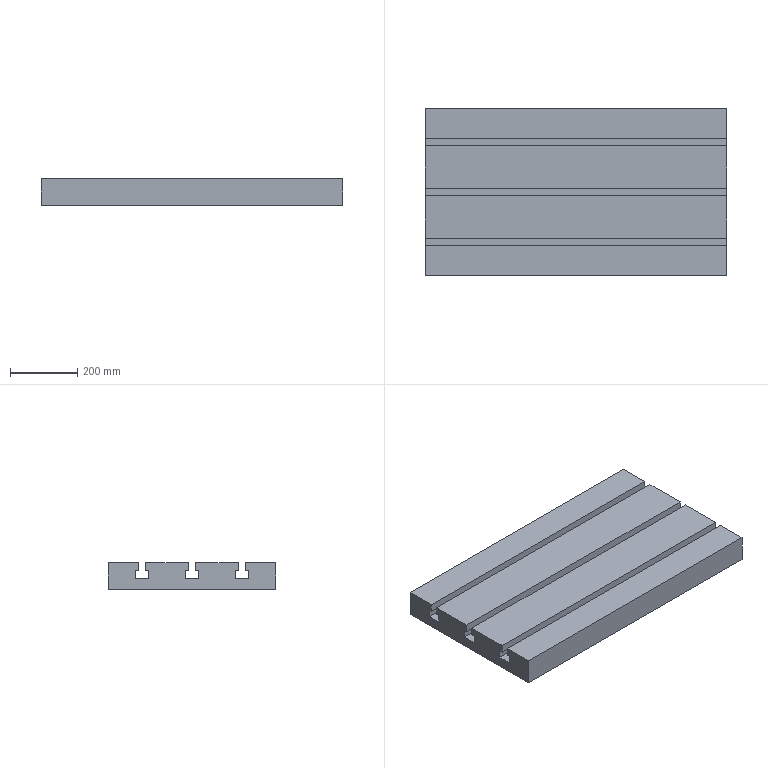Part | STEP file | 200 mesh_id2034 | 1 solid | 30 faces | box 900 x 500 x 80 mm | volume 31982400 mm3 | plane 30
STEP:
#1=CARTESIAN_POINT('',(-17333.884,-3882.269,-90.));
#2=VERTEX_POINT('',#1);
#3=CARTESIAN_POINT('',(-16433.884,-3882.269,-90.));
#4=VERTEX_POINT('',#3);
#5=CARTESIAN_POINT('',(-16423.884,-3882.269,-90.));
#6=DIRECTION('',(1.,0.,0.));
#7=VECTOR('',#6,1.);
#8=LINE('',#5,#7);
#9=EDGE_CURVE('',#2,#4,#8,.T.);
#10=ORIENTED_EDGE('',*,*,#9,.F.);
#11=CARTESIAN_POINT('',(-17333.884,-4009.269,-90.));
#12=VERTEX_POINT('',#11);
#13=CARTESIAN_POINT('',(-17333.884,-4020.269,-90.));
#14=DIRECTION('',(0.,1.,0.));
#15=VECTOR('',#14,1.);
#16=LINE('',#13,#15);
#17=EDGE_CURVE('',#12,#2,#16,.T.);
#18=ORIENTED_EDGE('',*,*,#17,.F.);
#19=CARTESIAN_POINT('',(-16433.884,-4009.269,-90.));
#20=VERTEX_POINT('',#19);
#21=CARTESIAN_POINT('',(-16423.884,-4009.269,-90.));
#22=DIRECTION('',(-1.,0.,0.));
#23=VECTOR('',#22,1.);
#24=LINE('',#21,#23);
#25=EDGE_CURVE('',#20,#12,#24,.T.);
#26=ORIENTED_EDGE('',*,*,#25,.F.);
#27=CARTESIAN_POINT('',(-16433.884,-4020.269,-90.));
#28=DIRECTION('',(0.,-1.,0.));
#29=VECTOR('',#28,1.);
#30=LINE('',#27,#29);
#31=EDGE_CURVE('',#4,#20,#30,.T.);
#32=ORIENTED_EDGE('',*,*,#31,.F.);
#33=EDGE_LOOP('',(#10,#18,#26,#32));
#34=FACE_OUTER_BOUND('',#33,.T.);
#35=CARTESIAN_POINT('',(-16883.884,-4020.269,-90.));
#36=DIRECTION('',(0.,0.,1.));
#37=DIRECTION('',(1.,0.,0.));
#38=AXIS2_PLACEMENT_3D('',#35,#36,#37);
#39=PLANE('',#38);
#40=ADVANCED_FACE('',(#34),#39,.T.);
#41=CARTESIAN_POINT('',(-17333.884,-3851.269,-114.));
#42=VERTEX_POINT('',#41);
#43=CARTESIAN_POINT('',(-17333.884,-3860.269,-114.));
#44=VERTEX_POINT('',#43);
#45=CARTESIAN_POINT('',(-17333.884,-4020.269,-114.));
#46=DIRECTION('',(0.,-1.,0.));
#47=VECTOR('',#46,1.);
#48=LINE('',#45,#47);
#49=EDGE_CURVE('',#42,#44,#48,.T.);
#50=ORIENTED_EDGE('',*,*,#49,.T.);
#51=CARTESIAN_POINT('',(-17333.884,-3860.269,-90.));
#52=VERTEX_POINT('',#51);
#53=CARTESIAN_POINT('',(-17333.884,-3860.269,-170.));
#54=DIRECTION('',(0.,0.,1.));
#55=VECTOR('',#54,1.);
#56=LINE('',#53,#55);
#57=EDGE_CURVE('',#44,#52,#56,.T.);
#58=ORIENTED_EDGE('',*,*,#57,.T.);
#59=CARTESIAN_POINT('',(-17333.884,-3770.269,-90.));
#60=VERTEX_POINT('',#59);
#61=CARTESIAN_POINT('',(-17333.884,-4020.269,-90.));
#62=DIRECTION('',(0.,1.,0.));
#63=VECTOR('',#62,1.);
#64=LINE('',#61,#63);
#65=EDGE_CURVE('',#52,#60,#64,.T.);
#66=ORIENTED_EDGE('',*,*,#65,.T.);
#67=CARTESIAN_POINT('',(-17333.884,-3770.269,-170.));
#68=VERTEX_POINT('',#67);
#69=CARTESIAN_POINT('',(-17333.884,-3770.269,-170.));
#70=DIRECTION('',(0.,0.,1.));
#71=VECTOR('',#70,1.);
#72=LINE('',#69,#71);
#73=EDGE_CURVE('',#68,#60,#72,.T.);
#74=ORIENTED_EDGE('',*,*,#73,.F.);
#75=CARTESIAN_POINT('',(-17333.884,-4270.269,-170.));
#76=VERTEX_POINT('',#75);
#77=CARTESIAN_POINT('',(-17333.884,-4020.269,-170.));
#78=DIRECTION('',(0.,-1.,0.));
#79=VECTOR('',#78,1.);
#80=LINE('',#77,#79);
#81=EDGE_CURVE('',#68,#76,#80,.T.);
#82=ORIENTED_EDGE('',*,*,#81,.T.);
#83=CARTESIAN_POINT('',(-17333.884,-4270.269,-90.));
#84=VERTEX_POINT('',#83);
#85=CARTESIAN_POINT('',(-17333.884,-4270.269,-170.));
#86=DIRECTION('',(0.,0.,1.));
#87=VECTOR('',#86,1.);
#88=LINE('',#85,#87);
#89=EDGE_CURVE('',#76,#84,#88,.T.);
#90=ORIENTED_EDGE('',*,*,#89,.T.);
#91=CARTESIAN_POINT('',(-17333.884,-4180.269,-90.));
#92=VERTEX_POINT('',#91);
#93=CARTESIAN_POINT('',(-17333.884,-4020.269,-90.));
#94=DIRECTION('',(0.,1.,0.));
#95=VECTOR('',#94,1.);
#96=LINE('',#93,#95);
#97=EDGE_CURVE('',#84,#92,#96,.T.);
#98=ORIENTED_EDGE('',*,*,#97,.T.);
#99=CARTESIAN_POINT('',(-17333.884,-4180.269,-114.));
#100=VERTEX_POINT('',#99);
#101=CARTESIAN_POINT('',(-17333.884,-4180.269,-170.));
#102=DIRECTION('',(0.,0.,-1.));
#103=VECTOR('',#102,1.);
#104=LINE('',#101,#103);
#105=EDGE_CURVE('',#92,#100,#104,.T.);
#106=ORIENTED_EDGE('',*,*,#105,.T.);
#107=CARTESIAN_POINT('',(-17333.884,-4189.269,-114.));
#108=VERTEX_POINT('',#107);
#109=CARTESIAN_POINT('',(-17333.884,-4020.269,-114.));
#110=DIRECTION('',(0.,-1.,0.));
#111=VECTOR('',#110,1.);
#112=LINE('',#109,#111);
#113=EDGE_CURVE('',#100,#108,#112,.T.);
#114=ORIENTED_EDGE('',*,*,#113,.T.);
#115=CARTESIAN_POINT('',(-17333.884,-4189.269,-138.));
#116=VERTEX_POINT('',#115);
#117=CARTESIAN_POINT('',(-17333.884,-4189.269,-170.));
#118=DIRECTION('',(0.,0.,-1.));
#119=VECTOR('',#118,1.);
#120=LINE('',#117,#119);
#121=EDGE_CURVE('',#108,#116,#120,.T.);
#122=ORIENTED_EDGE('',*,*,#121,.T.);
#123=CARTESIAN_POINT('',(-17333.884,-4149.269,-138.));
#124=VERTEX_POINT('',#123);
#125=CARTESIAN_POINT('',(-17333.884,-4020.269,-138.));
#126=DIRECTION('',(0.,1.,0.));
#127=VECTOR('',#126,1.);
#128=LINE('',#125,#127);
#129=EDGE_CURVE('',#116,#124,#128,.T.);
#130=ORIENTED_EDGE('',*,*,#129,.T.);
#131=CARTESIAN_POINT('',(-17333.884,-4149.269,-114.));
#132=VERTEX_POINT('',#131);
#133=CARTESIAN_POINT('',(-17333.884,-4149.269,-170.));
#134=DIRECTION('',(0.,0.,1.));
#135=VECTOR('',#134,1.);
#136=LINE('',#133,#135);
#137=EDGE_CURVE('',#124,#132,#136,.T.);
#138=ORIENTED_EDGE('',*,*,#137,.T.);
#139=CARTESIAN_POINT('',(-17333.884,-4158.269,-114.));
#140=VERTEX_POINT('',#139);
#141=CARTESIAN_POINT('',(-17333.884,-4020.269,-114.));
#142=DIRECTION('',(0.,-1.,0.));
#143=VECTOR('',#142,1.);
#144=LINE('',#141,#143);
#145=EDGE_CURVE('',#132,#140,#144,.T.);
#146=ORIENTED_EDGE('',*,*,#145,.T.);
#147=CARTESIAN_POINT('',(-17333.884,-4158.269,-90.));
#148=VERTEX_POINT('',#147);
#149=CARTESIAN_POINT('',(-17333.884,-4158.269,-170.));
#150=DIRECTION('',(0.,0.,1.));
#151=VECTOR('',#150,1.);
#152=LINE('',#149,#151);
#153=EDGE_CURVE('',#140,#148,#152,.T.);
#154=ORIENTED_EDGE('',*,*,#153,.T.);
#155=CARTESIAN_POINT('',(-17333.884,-4031.269,-90.));
#156=VERTEX_POINT('',#155);
#157=CARTESIAN_POINT('',(-17333.884,-4020.269,-90.));
#158=DIRECTION('',(0.,1.,0.));
#159=VECTOR('',#158,1.);
#160=LINE('',#157,#159);
#161=EDGE_CURVE('',#148,#156,#160,.T.);
#162=ORIENTED_EDGE('',*,*,#161,.T.);
#163=CARTESIAN_POINT('',(-17333.884,-4031.269,-114.));
#164=VERTEX_POINT('',#163);
#165=CARTESIAN_POINT('',(-17333.884,-4031.269,-170.));
#166=DIRECTION('',(0.,0.,-1.));
#167=VECTOR('',#166,1.);
#168=LINE('',#165,#167);
#169=EDGE_CURVE('',#156,#164,#168,.T.);
#170=ORIENTED_EDGE('',*,*,#169,.T.);
#171=CARTESIAN_POINT('',(-17333.884,-4040.269,-114.));
#172=VERTEX_POINT('',#171);
#173=CARTESIAN_POINT('',(-17333.884,-4020.269,-114.));
#174=DIRECTION('',(0.,-1.,0.));
#175=VECTOR('',#174,1.);
#176=LINE('',#173,#175);
#177=EDGE_CURVE('',#164,#172,#176,.T.);
#178=ORIENTED_EDGE('',*,*,#177,.T.);
#179=CARTESIAN_POINT('',(-17333.884,-4040.269,-138.));
#180=VERTEX_POINT('',#179);
#181=CARTESIAN_POINT('',(-17333.884,-4040.269,-170.));
#182=DIRECTION('',(0.,0.,-1.));
#183=VECTOR('',#182,1.);
#184=LINE('',#181,#183);
#185=EDGE_CURVE('',#172,#180,#184,.T.);
#186=ORIENTED_EDGE('',*,*,#185,.T.);
#187=CARTESIAN_POINT('',(-17333.884,-4000.269,-138.));
#188=VERTEX_POINT('',#187);
#189=CARTESIAN_POINT('',(-17333.884,-4020.269,-138.));
#190=DIRECTION('',(0.,1.,0.));
#191=VECTOR('',#190,1.);
#192=LINE('',#189,#191);
#193=EDGE_CURVE('',#180,#188,#192,.T.);
#194=ORIENTED_EDGE('',*,*,#193,.T.);
#195=CARTESIAN_POINT('',(-17333.884,-4000.269,-114.));
#196=VERTEX_POINT('',#195);
#197=CARTESIAN_POINT('',(-17333.884,-4000.269,-170.));
#198=DIRECTION('',(0.,0.,1.));
#199=VECTOR('',#198,1.);
#200=LINE('',#197,#199);
#201=EDGE_CURVE('',#188,#196,#200,.T.);
#202=ORIENTED_EDGE('',*,*,#201,.T.);
#203=CARTESIAN_POINT('',(-17333.884,-4009.269,-114.));
#204=VERTEX_POINT('',#203);
#205=CARTESIAN_POINT('',(-17333.884,-4020.269,-114.));
#206=DIRECTION('',(0.,-1.,0.));
#207=VECTOR('',#206,1.);
#208=LINE('',#205,#207);
#209=EDGE_CURVE('',#196,#204,#208,.T.);
#210=ORIENTED_EDGE('',*,*,#209,.T.);
#211=CARTESIAN_POINT('',(-17333.884,-4009.269,-170.));
#212=DIRECTION('',(0.,0.,1.));
#213=VECTOR('',#212,1.);
#214=LINE('',#211,#213);
#215=EDGE_CURVE('',#204,#12,#214,.T.);
#216=ORIENTED_EDGE('',*,*,#215,.T.);
#217=ORIENTED_EDGE('',*,*,#17,.T.);
#218=CARTESIAN_POINT('',(-17333.884,-3882.269,-114.));
#219=VERTEX_POINT('',#218);
#220=CARTESIAN_POINT('',(-17333.884,-3882.269,-170.));
#221=DIRECTION('',(0.,0.,-1.));
#222=VECTOR('',#221,1.);
#223=LINE('',#220,#222);
#224=EDGE_CURVE('',#2,#219,#223,.T.);
#225=ORIENTED_EDGE('',*,*,#224,.T.);
#226=CARTESIAN_POINT('',(-17333.884,-3891.269,-114.));
#227=VERTEX_POINT('',#226);
#228=CARTESIAN_POINT('',(-17333.884,-4020.269,-114.));
#229=DIRECTION('',(0.,-1.,0.));
#230=VECTOR('',#229,1.);
#231=LINE('',#228,#230);
#232=EDGE_CURVE('',#219,#227,#231,.T.);
#233=ORIENTED_EDGE('',*,*,#232,.T.);
#234=CARTESIAN_POINT('',(-17333.884,-3891.269,-138.));
#235=VERTEX_POINT('',#234);
#236=CARTESIAN_POINT('',(-17333.884,-3891.269,-170.));
#237=DIRECTION('',(0.,0.,-1.));
#238=VECTOR('',#237,1.);
#239=LINE('',#236,#238);
#240=EDGE_CURVE('',#227,#235,#239,.T.);
#241=ORIENTED_EDGE('',*,*,#240,.T.);
#242=CARTESIAN_POINT('',(-17333.884,-3851.269,-138.));
#243=VERTEX_POINT('',#242);
#244=CARTESIAN_POINT('',(-17333.884,-4020.269,-138.));
#245=DIRECTION('',(0.,1.,0.));
#246=VECTOR('',#245,1.);
#247=LINE('',#244,#246);
#248=EDGE_CURVE('',#235,#243,#247,.T.);
#249=ORIENTED_EDGE('',*,*,#248,.T.);
#250=CARTESIAN_POINT('',(-17333.884,-3851.269,-170.));
#251=DIRECTION('',(0.,0.,1.));
#252=VECTOR('',#251,1.);
#253=LINE('',#250,#252);
#254=EDGE_CURVE('',#243,#42,#253,.T.);
#255=ORIENTED_EDGE('',*,*,#254,.T.);
#256=EDGE_LOOP('',(#50,#58,#66,#74,#82,#90,#98,#106,#114,#122,#130,#138,#146,#154,#162,#170,#178,#186,#194,#202,#210,#216,#217,#225,#233,#241,#249,#255));
#257=FACE_OUTER_BOUND('',#256,.T.);
#258=CARTESIAN_POINT('',(-17333.884,-4020.269,-170.));
#259=DIRECTION('',(-1.,0.,0.));
#260=DIRECTION('',(0.,0.,1.));
#261=AXIS2_PLACEMENT_3D('',#258,#259,#260);
#262=PLANE('',#261);
#263=ADVANCED_FACE('',(#257),#262,.T.);
#264=CARTESIAN_POINT('',(-16433.884,-3770.269,-90.));
#265=VERTEX_POINT('',#264);
#266=CARTESIAN_POINT('',(-16433.884,-3860.269,-90.));
#267=VERTEX_POINT('',#266);
#268=CARTESIAN_POINT('',(-16433.884,-4020.269,-90.));
#269=DIRECTION('',(0.,-1.,0.));
#270=VECTOR('',#269,1.);
#271=LINE('',#268,#270);
#272=EDGE_CURVE('',#265,#267,#271,.T.);
#273=ORIENTED_EDGE('',*,*,#272,.T.);
#274=CARTESIAN_POINT('',(-16433.884,-3860.269,-114.));
#275=VERTEX_POINT('',#274);
#276=CARTESIAN_POINT('',(-16433.884,-3860.269,-170.));
#277=DIRECTION('',(0.,0.,-1.));
#278=VECTOR('',#277,1.);
#279=LINE('',#276,#278);
#280=EDGE_CURVE('',#267,#275,#279,.T.);
#281=ORIENTED_EDGE('',*,*,#280,.T.);
#282=CARTESIAN_POINT('',(-16433.884,-3851.269,-114.));
#283=VERTEX_POINT('',#282);
#284=CARTESIAN_POINT('',(-16433.884,-4020.269,-114.));
#285=DIRECTION('',(0.,1.,0.));
#286=VECTOR('',#285,1.);
#287=LINE('',#284,#286);
#288=EDGE_CURVE('',#275,#283,#287,.T.);
#289=ORIENTED_EDGE('',*,*,#288,.T.);
#290=CARTESIAN_POINT('',(-16433.884,-3851.269,-138.));
#291=VERTEX_POINT('',#290);
#292=CARTESIAN_POINT('',(-16433.884,-3851.269,-170.));
#293=DIRECTION('',(0.,0.,-1.));
#294=VECTOR('',#293,1.);
#295=LINE('',#292,#294);
#296=EDGE_CURVE('',#283,#291,#295,.T.);
#297=ORIENTED_EDGE('',*,*,#296,.T.);
#298=CARTESIAN_POINT('',(-16433.884,-3891.269,-138.));
#299=VERTEX_POINT('',#298);
#300=CARTESIAN_POINT('',(-16433.884,-4020.269,-138.));
#301=DIRECTION('',(0.,-1.,0.));
#302=VECTOR('',#301,1.);
#303=LINE('',#300,#302);
#304=EDGE_CURVE('',#291,#299,#303,.T.);
#305=ORIENTED_EDGE('',*,*,#304,.T.);
#306=CARTESIAN_POINT('',(-16433.884,-3891.269,-114.));
#307=VERTEX_POINT('',#306);
#308=CARTESIAN_POINT('',(-16433.884,-3891.269,-170.));
#309=DIRECTION('',(0.,0.,1.));
#310=VECTOR('',#309,1.);
#311=LINE('',#308,#310);
#312=EDGE_CURVE('',#299,#307,#311,.T.);
#313=ORIENTED_EDGE('',*,*,#312,.T.);
#314=CARTESIAN_POINT('',(-16433.884,-3882.269,-114.));
#315=VERTEX_POINT('',#314);
#316=CARTESIAN_POINT('',(-16433.884,-4020.269,-114.));
#317=DIRECTION('',(0.,1.,0.));
#318=VECTOR('',#317,1.);
#319=LINE('',#316,#318);
#320=EDGE_CURVE('',#307,#315,#319,.T.);
#321=ORIENTED_EDGE('',*,*,#320,.T.);
#322=CARTESIAN_POINT('',(-16433.884,-3882.269,-170.));
#323=DIRECTION('',(0.,0.,1.));
#324=VECTOR('',#323,1.);
#325=LINE('',#322,#324);
#326=EDGE_CURVE('',#315,#4,#325,.T.);
#327=ORIENTED_EDGE('',*,*,#326,.T.);
#328=ORIENTED_EDGE('',*,*,#31,.T.);
#329=CARTESIAN_POINT('',(-16433.884,-4009.269,-114.));
#330=VERTEX_POINT('',#329);
#331=CARTESIAN_POINT('',(-16433.884,-4009.269,-170.));
#332=DIRECTION('',(0.,0.,-1.));
#333=VECTOR('',#332,1.);
#334=LINE('',#331,#333);
#335=EDGE_CURVE('',#20,#330,#334,.T.);
#336=ORIENTED_EDGE('',*,*,#335,.T.);
#337=CARTESIAN_POINT('',(-16433.884,-4000.269,-114.));
#338=VERTEX_POINT('',#337);
#339=CARTESIAN_POINT('',(-16433.884,-4020.269,-114.));
#340=DIRECTION('',(0.,1.,0.));
#341=VECTOR('',#340,1.);
#342=LINE('',#339,#341);
#343=EDGE_CURVE('',#330,#338,#342,.T.);
#344=ORIENTED_EDGE('',*,*,#343,.T.);
#345=CARTESIAN_POINT('',(-16433.884,-4000.269,-138.));
#346=VERTEX_POINT('',#345);
#347=CARTESIAN_POINT('',(-16433.884,-4000.269,-170.));
#348=DIRECTION('',(0.,0.,-1.));
#349=VECTOR('',#348,1.);
#350=LINE('',#347,#349);
#351=EDGE_CURVE('',#338,#346,#350,.T.);
#352=ORIENTED_EDGE('',*,*,#351,.T.);
#353=CARTESIAN_POINT('',(-16433.884,-4040.269,-138.));
#354=VERTEX_POINT('',#353);
#355=CARTESIAN_POINT('',(-16433.884,-4020.269,-138.));
#356=DIRECTION('',(0.,-1.,0.));
#357=VECTOR('',#356,1.);
#358=LINE('',#355,#357);
#359=EDGE_CURVE('',#346,#354,#358,.T.);
#360=ORIENTED_EDGE('',*,*,#359,.T.);
#361=CARTESIAN_POINT('',(-16433.884,-4040.269,-114.));
#362=VERTEX_POINT('',#361);
#363=CARTESIAN_POINT('',(-16433.884,-4040.269,-170.));
#364=DIRECTION('',(0.,0.,1.));
#365=VECTOR('',#364,1.);
#366=LINE('',#363,#365);
#367=EDGE_CURVE('',#354,#362,#366,.T.);
#368=ORIENTED_EDGE('',*,*,#367,.T.);
#369=CARTESIAN_POINT('',(-16433.884,-4031.269,-114.));
#370=VERTEX_POINT('',#369);
#371=CARTESIAN_POINT('',(-16433.884,-4020.269,-114.));
#372=DIRECTION('',(0.,1.,0.));
#373=VECTOR('',#372,1.);
#374=LINE('',#371,#373);
#375=EDGE_CURVE('',#362,#370,#374,.T.);
#376=ORIENTED_EDGE('',*,*,#375,.T.);
#377=CARTESIAN_POINT('',(-16433.884,-4031.269,-90.));
#378=VERTEX_POINT('',#377);
#379=CARTESIAN_POINT('',(-16433.884,-4031.269,-170.));
#380=DIRECTION('',(0.,0.,1.));
#381=VECTOR('',#380,1.);
#382=LINE('',#379,#381);
#383=EDGE_CURVE('',#370,#378,#382,.T.);
#384=ORIENTED_EDGE('',*,*,#383,.T.);
#385=CARTESIAN_POINT('',(-16433.884,-4158.269,-90.));
#386=VERTEX_POINT('',#385);
#387=CARTESIAN_POINT('',(-16433.884,-4020.269,-90.));
#388=DIRECTION('',(0.,-1.,0.));
#389=VECTOR('',#388,1.);
#390=LINE('',#387,#389);
#391=EDGE_CURVE('',#378,#386,#390,.T.);
#392=ORIENTED_EDGE('',*,*,#391,.T.);
#393=CARTESIAN_POINT('',(-16433.884,-4158.269,-114.));
#394=VERTEX_POINT('',#393);
#395=CARTESIAN_POINT('',(-16433.884,-4158.269,-170.));
#396=DIRECTION('',(0.,0.,-1.));
#397=VECTOR('',#396,1.);
#398=LINE('',#395,#397);
#399=EDGE_CURVE('',#386,#394,#398,.T.);
#400=ORIENTED_EDGE('',*,*,#399,.T.);
#401=CARTESIAN_POINT('',(-16433.884,-4149.269,-114.));
#402=VERTEX_POINT('',#401);
#403=CARTESIAN_POINT('',(-16433.884,-4020.269,-114.));
#404=DIRECTION('',(0.,1.,0.));
#405=VECTOR('',#404,1.);
#406=LINE('',#403,#405);
#407=EDGE_CURVE('',#394,#402,#406,.T.);
#408=ORIENTED_EDGE('',*,*,#407,.T.);
#409=CARTESIAN_POINT('',(-16433.884,-4149.269,-138.));
#410=VERTEX_POINT('',#409);
#411=CARTESIAN_POINT('',(-16433.884,-4149.269,-170.));
#412=DIRECTION('',(0.,0.,-1.));
#413=VECTOR('',#412,1.);
#414=LINE('',#411,#413);
#415=EDGE_CURVE('',#402,#410,#414,.T.);
#416=ORIENTED_EDGE('',*,*,#415,.T.);
#417=CARTESIAN_POINT('',(-16433.884,-4189.269,-138.));
#418=VERTEX_POINT('',#417);
#419=CARTESIAN_POINT('',(-16433.884,-4020.269,-138.));
#420=DIRECTION('',(0.,-1.,0.));
#421=VECTOR('',#420,1.);
#422=LINE('',#419,#421);
#423=EDGE_CURVE('',#410,#418,#422,.T.);
#424=ORIENTED_EDGE('',*,*,#423,.T.);
#425=CARTESIAN_POINT('',(-16433.884,-4189.269,-114.));
#426=VERTEX_POINT('',#425);
#427=CARTESIAN_POINT('',(-16433.884,-4189.269,-170.));
#428=DIRECTION('',(0.,0.,1.));
#429=VECTOR('',#428,1.);
#430=LINE('',#427,#429);
#431=EDGE_CURVE('',#418,#426,#430,.T.);
#432=ORIENTED_EDGE('',*,*,#431,.T.);
#433=CARTESIAN_POINT('',(-16433.884,-4180.269,-114.));
#434=VERTEX_POINT('',#433);
#435=CARTESIAN_POINT('',(-16433.884,-4020.269,-114.));
#436=DIRECTION('',(0.,1.,0.));
#437=VECTOR('',#436,1.);
#438=LINE('',#435,#437);
#439=EDGE_CURVE('',#426,#434,#438,.T.);
#440=ORIENTED_EDGE('',*,*,#439,.T.);
#441=CARTESIAN_POINT('',(-16433.884,-4180.269,-90.));
#442=VERTEX_POINT('',#441);
#443=CARTESIAN_POINT('',(-16433.884,-4180.269,-170.));
#444=DIRECTION('',(0.,0.,1.));
#445=VECTOR('',#444,1.);
#446=LINE('',#443,#445);
#447=EDGE_CURVE('',#434,#442,#446,.T.);
#448=ORIENTED_EDGE('',*,*,#447,.T.);
#449=CARTESIAN_POINT('',(-16433.884,-4270.269,-90.));
#450=VERTEX_POINT('',#449);
#451=CARTESIAN_POINT('',(-16433.884,-4020.269,-90.));
#452=DIRECTION('',(0.,-1.,0.));
#453=VECTOR('',#452,1.);
#454=LINE('',#451,#453);
#455=EDGE_CURVE('',#442,#450,#454,.T.);
#456=ORIENTED_EDGE('',*,*,#455,.T.);
#457=CARTESIAN_POINT('',(-16433.884,-4270.269,-170.));
#458=VERTEX_POINT('',#457);
#459=CARTESIAN_POINT('',(-16433.884,-4270.269,-170.));
#460=DIRECTION('',(0.,0.,1.));
#461=VECTOR('',#460,1.);
#462=LINE('',#459,#461);
#463=EDGE_CURVE('',#458,#450,#462,.T.);
#464=ORIENTED_EDGE('',*,*,#463,.F.);
#465=CARTESIAN_POINT('',(-16433.884,-3770.269,-170.));
#466=VERTEX_POINT('',#465);
#467=CARTESIAN_POINT('',(-16433.884,-4020.269,-170.));
#468=DIRECTION('',(0.,1.,0.));
#469=VECTOR('',#468,1.);
#470=LINE('',#467,#469);
#471=EDGE_CURVE('',#458,#466,#470,.T.);
#472=ORIENTED_EDGE('',*,*,#471,.T.);
#473=CARTESIAN_POINT('',(-16433.884,-3770.269,-170.));
#474=DIRECTION('',(0.,0.,1.));
#475=VECTOR('',#474,1.);
#476=LINE('',#473,#475);
#477=EDGE_CURVE('',#466,#265,#476,.T.);
#478=ORIENTED_EDGE('',*,*,#477,.T.);
#479=EDGE_LOOP('',(#273,#281,#289,#297,#305,#313,#321,#327,#328,#336,#344,#352,#360,#368,#376,#384,#392,#400,#408,#416,#424,#432,#440,#448,#456,#464,#472,#478));
#480=FACE_OUTER_BOUND('',#479,.T.);
#481=CARTESIAN_POINT('',(-16433.884,-4020.269,-170.));
#482=DIRECTION('',(1.,0.,0.));
#483=DIRECTION('',(0.,0.,-1.));
#484=AXIS2_PLACEMENT_3D('',#481,#482,#483);
#485=PLANE('',#484);
#486=ADVANCED_FACE('',(#480),#485,.T.);
#487=CARTESIAN_POINT('',(-16423.884,-3860.269,-90.));
#488=DIRECTION('',(-1.,0.,0.));
#489=VECTOR('',#488,1.);
#490=LINE('',#487,#489);
#491=EDGE_CURVE('',#267,#52,#490,.T.);
#492=ORIENTED_EDGE('',*,*,#491,.F.);
#493=ORIENTED_EDGE('',*,*,#272,.F.);
#494=CARTESIAN_POINT('',(-16883.884,-3770.269,-90.));
#495=DIRECTION('',(1.,0.,0.));
#496=VECTOR('',#495,1.);
#497=LINE('',#494,#496);
#498=EDGE_CURVE('',#60,#265,#497,.T.);
#499=ORIENTED_EDGE('',*,*,#498,.F.);
#500=ORIENTED_EDGE('',*,*,#65,.F.);
#501=EDGE_LOOP('',(#492,#493,#499,#500));
#502=FACE_OUTER_BOUND('',#501,.T.);
#503=CARTESIAN_POINT('',(-16883.884,-4020.269,-90.));
#504=DIRECTION('',(0.,0.,1.));
#505=DIRECTION('',(1.,0.,0.));
#506=AXIS2_PLACEMENT_3D('',#503,#504,#505);
#507=PLANE('',#506);
#508=ADVANCED_FACE('',(#502),#507,.T.);
#509=CARTESIAN_POINT('',(-16423.884,-4031.269,-90.));
#510=DIRECTION('',(1.,0.,0.));
#511=VECTOR('',#510,1.);
#512=LINE('',#509,#511);
#513=EDGE_CURVE('',#156,#378,#512,.T.);
#514=ORIENTED_EDGE('',*,*,#513,.F.);
#515=ORIENTED_EDGE('',*,*,#161,.F.);
#516=CARTESIAN_POINT('',(-16423.884,-4158.269,-90.));
#517=DIRECTION('',(-1.,0.,0.));
#518=VECTOR('',#517,1.);
#519=LINE('',#516,#518);
#520=EDGE_CURVE('',#386,#148,#519,.T.);
#521=ORIENTED_EDGE('',*,*,#520,.F.);
#522=ORIENTED_EDGE('',*,*,#391,.F.);
#523=EDGE_LOOP('',(#514,#515,#521,#522));
#524=FACE_OUTER_BOUND('',#523,.T.);
#525=CARTESIAN_POINT('',(-16883.884,-4020.269,-90.));
#526=DIRECTION('',(0.,0.,1.));
#527=DIRECTION('',(1.,0.,0.));
#528=AXIS2_PLACEMENT_3D('',#525,#526,#527);
#529=PLANE('',#528);
#530=ADVANCED_FACE('',(#524),#529,.T.);
#531=CARTESIAN_POINT('',(-16423.884,-4180.269,-90.));
#532=DIRECTION('',(1.,0.,0.));
#533=VECTOR('',#532,1.);
#534=LINE('',#531,#533);
#535=EDGE_CURVE('',#92,#442,#534,.T.);
#536=ORIENTED_EDGE('',*,*,#535,.F.);
#537=ORIENTED_EDGE('',*,*,#97,.F.);
#538=CARTESIAN_POINT('',(-16883.884,-4270.269,-90.));
#539=DIRECTION('',(-1.,0.,0.));
#540=VECTOR('',#539,1.);
#541=LINE('',#538,#540);
#542=EDGE_CURVE('',#450,#84,#541,.T.);
#543=ORIENTED_EDGE('',*,*,#542,.F.);
#544=ORIENTED_EDGE('',*,*,#455,.F.);
#545=EDGE_LOOP('',(#536,#537,#543,#544));
#546=FACE_OUTER_BOUND('',#545,.T.);
#547=CARTESIAN_POINT('',(-16883.884,-4020.269,-90.));
#548=DIRECTION('',(0.,0.,1.));
#549=DIRECTION('',(1.,0.,0.));
#550=AXIS2_PLACEMENT_3D('',#547,#548,#549);
#551=PLANE('',#550);
#552=ADVANCED_FACE('',(#546),#551,.T.);
#553=ORIENTED_EDGE('',*,*,#463,.T.);
#554=ORIENTED_EDGE('',*,*,#542,.T.);
#555=ORIENTED_EDGE('',*,*,#89,.F.);
#556=CARTESIAN_POINT('',(-16883.884,-4270.269,-170.));
#557=DIRECTION('',(1.,0.,0.));
#558=VECTOR('',#557,1.);
#559=LINE('',#556,#558);
#560=EDGE_CURVE('',#76,#458,#559,.T.);
#561=ORIENTED_EDGE('',*,*,#560,.T.);
#562=EDGE_LOOP('',(#553,#554,#555,#561));
#563=FACE_OUTER_BOUND('',#562,.T.);
#564=CARTESIAN_POINT('',(-16883.884,-4270.269,-170.));
#565=DIRECTION('',(0.,-1.,0.));
#566=DIRECTION('',(0.,0.,-1.));
#567=AXIS2_PLACEMENT_3D('',#564,#565,#566);
#568=PLANE('',#567);
#569=ADVANCED_FACE('',(#563),#568,.T.);
#570=ORIENTED_EDGE('',*,*,#73,.T.);
#571=ORIENTED_EDGE('',*,*,#498,.T.);
#572=ORIENTED_EDGE('',*,*,#477,.F.);
#573=CARTESIAN_POINT('',(-16883.884,-3770.269,-170.));
#574=DIRECTION('',(-1.,0.,0.));
#575=VECTOR('',#574,1.);
#576=LINE('',#573,#575);
#577=EDGE_CURVE('',#466,#68,#576,.T.);
#578=ORIENTED_EDGE('',*,*,#577,.T.);
#579=EDGE_LOOP('',(#570,#571,#572,#578));
#580=FACE_OUTER_BOUND('',#579,.T.);
#581=CARTESIAN_POINT('',(-16883.884,-3770.269,-170.));
#582=DIRECTION('',(0.,1.,0.));
#583=DIRECTION('',(0.,0.,1.));
#584=AXIS2_PLACEMENT_3D('',#581,#582,#583);
#585=PLANE('',#584);
#586=ADVANCED_FACE('',(#580),#585,.T.);
#587=ORIENTED_EDGE('',*,*,#471,.F.);
#588=ORIENTED_EDGE('',*,*,#560,.F.);
#589=ORIENTED_EDGE('',*,*,#81,.F.);
#590=ORIENTED_EDGE('',*,*,#577,.F.);
#591=EDGE_LOOP('',(#587,#588,#589,#590));
#592=FACE_OUTER_BOUND('',#591,.T.);
#593=CARTESIAN_POINT('',(-16883.884,-4020.269,-170.));
#594=DIRECTION('',(0.,0.,-1.));
#595=DIRECTION('',(-1.,0.,0.));
#596=AXIS2_PLACEMENT_3D('',#593,#594,#595);
#597=PLANE('',#596);
#598=ADVANCED_FACE('',(#592),#597,.T.);
#599=ORIENTED_EDGE('',*,*,#153,.F.);
#600=CARTESIAN_POINT('',(-16423.884,-4158.269,-114.));
#601=DIRECTION('',(-1.,0.,0.));
#602=VECTOR('',#601,1.);
#603=LINE('',#600,#602);
#604=EDGE_CURVE('',#394,#140,#603,.T.);
#605=ORIENTED_EDGE('',*,*,#604,.F.);
#606=ORIENTED_EDGE('',*,*,#399,.F.);
#607=ORIENTED_EDGE('',*,*,#520,.T.);
#608=EDGE_LOOP('',(#599,#605,#606,#607));
#609=FACE_OUTER_BOUND('',#608,.T.);
#610=CARTESIAN_POINT('',(-16423.884,-4158.269,-114.));
#611=DIRECTION('',(0.,-1.,0.));
#612=DIRECTION('',(0.,0.,-1.));
#613=AXIS2_PLACEMENT_3D('',#610,#611,#612);
#614=PLANE('',#613);
#615=ADVANCED_FACE('',(#609),#614,.T.);
#616=ORIENTED_EDGE('',*,*,#145,.F.);
#617=CARTESIAN_POINT('',(-16423.884,-4149.269,-114.));
#618=DIRECTION('',(-1.,0.,0.));
#619=VECTOR('',#618,1.);
#620=LINE('',#617,#619);
#621=EDGE_CURVE('',#402,#132,#620,.T.);
#622=ORIENTED_EDGE('',*,*,#621,.F.);
#623=ORIENTED_EDGE('',*,*,#407,.F.);
#624=ORIENTED_EDGE('',*,*,#604,.T.);
#625=EDGE_LOOP('',(#616,#622,#623,#624));
#626=FACE_OUTER_BOUND('',#625,.T.);
#627=CARTESIAN_POINT('',(-16423.884,-4149.269,-114.));
#628=DIRECTION('',(0.,0.,-1.));
#629=DIRECTION('',(-1.,0.,0.));
#630=AXIS2_PLACEMENT_3D('',#627,#628,#629);
#631=PLANE('',#630);
#632=ADVANCED_FACE('',(#626),#631,.T.);
#633=ORIENTED_EDGE('',*,*,#137,.F.);
#634=CARTESIAN_POINT('',(-16423.884,-4149.269,-138.));
#635=DIRECTION('',(-1.,0.,0.));
#636=VECTOR('',#635,1.);
#637=LINE('',#634,#636);
#638=EDGE_CURVE('',#410,#124,#637,.T.);
#639=ORIENTED_EDGE('',*,*,#638,.F.);
#640=ORIENTED_EDGE('',*,*,#415,.F.);
#641=ORIENTED_EDGE('',*,*,#621,.T.);
#642=EDGE_LOOP('',(#633,#639,#640,#641));
#643=FACE_OUTER_BOUND('',#642,.T.);
#644=CARTESIAN_POINT('',(-16423.884,-4149.269,-138.));
#645=DIRECTION('',(0.,-1.,0.));
#646=DIRECTION('',(0.,0.,-1.));
#647=AXIS2_PLACEMENT_3D('',#644,#645,#646);
#648=PLANE('',#647);
#649=ADVANCED_FACE('',(#643),#648,.T.);
#650=ORIENTED_EDGE('',*,*,#129,.F.);
#651=CARTESIAN_POINT('',(-16423.884,-4189.269,-138.));
#652=DIRECTION('',(-1.,0.,0.));
#653=VECTOR('',#652,1.);
#654=LINE('',#651,#653);
#655=EDGE_CURVE('',#418,#116,#654,.T.);
#656=ORIENTED_EDGE('',*,*,#655,.F.);
#657=ORIENTED_EDGE('',*,*,#423,.F.);
#658=ORIENTED_EDGE('',*,*,#638,.T.);
#659=EDGE_LOOP('',(#650,#656,#657,#658));
#660=FACE_OUTER_BOUND('',#659,.T.);
#661=CARTESIAN_POINT('',(-16423.884,-4189.269,-138.));
#662=DIRECTION('',(0.,0.,1.));
#663=DIRECTION('',(1.,0.,0.));
#664=AXIS2_PLACEMENT_3D('',#661,#662,#663);
#665=PLANE('',#664);
#666=ADVANCED_FACE('',(#660),#665,.T.);
#667=ORIENTED_EDGE('',*,*,#121,.F.);
#668=CARTESIAN_POINT('',(-16423.884,-4189.269,-114.));
#669=DIRECTION('',(-1.,0.,0.));
#670=VECTOR('',#669,1.);
#671=LINE('',#668,#670);
#672=EDGE_CURVE('',#426,#108,#671,.T.);
#673=ORIENTED_EDGE('',*,*,#672,.F.);
#674=ORIENTED_EDGE('',*,*,#431,.F.);
#675=ORIENTED_EDGE('',*,*,#655,.T.);
#676=EDGE_LOOP('',(#667,#673,#674,#675));
#677=FACE_OUTER_BOUND('',#676,.T.);
#678=CARTESIAN_POINT('',(-16423.884,-4189.269,-114.));
#679=DIRECTION('',(0.,1.,0.));
#680=DIRECTION('',(0.,0.,1.));
#681=AXIS2_PLACEMENT_3D('',#678,#679,#680);
#682=PLANE('',#681);
#683=ADVANCED_FACE('',(#677),#682,.T.);
#684=ORIENTED_EDGE('',*,*,#113,.F.);
#685=CARTESIAN_POINT('',(-16423.884,-4180.269,-114.));
#686=DIRECTION('',(-1.,0.,0.));
#687=VECTOR('',#686,1.);
#688=LINE('',#685,#687);
#689=EDGE_CURVE('',#434,#100,#688,.T.);
#690=ORIENTED_EDGE('',*,*,#689,.F.);
#691=ORIENTED_EDGE('',*,*,#439,.F.);
#692=ORIENTED_EDGE('',*,*,#672,.T.);
#693=EDGE_LOOP('',(#684,#690,#691,#692));
#694=FACE_OUTER_BOUND('',#693,.T.);
#695=CARTESIAN_POINT('',(-16423.884,-4180.269,-114.));
#696=DIRECTION('',(0.,0.,-1.));
#697=DIRECTION('',(-1.,0.,0.));
#698=AXIS2_PLACEMENT_3D('',#695,#696,#697);
#699=PLANE('',#698);
#700=ADVANCED_FACE('',(#694),#699,.T.);
#701=ORIENTED_EDGE('',*,*,#105,.F.);
#702=ORIENTED_EDGE('',*,*,#535,.T.);
#703=ORIENTED_EDGE('',*,*,#447,.F.);
#704=ORIENTED_EDGE('',*,*,#689,.T.);
#705=EDGE_LOOP('',(#701,#702,#703,#704));
#706=FACE_OUTER_BOUND('',#705,.T.);
#707=CARTESIAN_POINT('',(-16423.884,-4180.269,-90.));
#708=DIRECTION('',(0.,1.,0.));
#709=DIRECTION('',(0.,0.,1.));
#710=AXIS2_PLACEMENT_3D('',#707,#708,#709);
#711=PLANE('',#710);
#712=ADVANCED_FACE('',(#706),#711,.T.);
#713=ORIENTED_EDGE('',*,*,#215,.F.);
#714=CARTESIAN_POINT('',(-16423.884,-4009.269,-114.));
#715=DIRECTION('',(-1.,0.,0.));
#716=VECTOR('',#715,1.);
#717=LINE('',#714,#716);
#718=EDGE_CURVE('',#330,#204,#717,.T.);
#719=ORIENTED_EDGE('',*,*,#718,.F.);
#720=ORIENTED_EDGE('',*,*,#335,.F.);
#721=ORIENTED_EDGE('',*,*,#25,.T.);
#722=EDGE_LOOP('',(#713,#719,#720,#721));
#723=FACE_OUTER_BOUND('',#722,.T.);
#724=CARTESIAN_POINT('',(-16423.884,-4009.269,-114.));
#725=DIRECTION('',(0.,-1.,0.));
#726=DIRECTION('',(0.,0.,-1.));
#727=AXIS2_PLACEMENT_3D('',#724,#725,#726);
#728=PLANE('',#727);
#729=ADVANCED_FACE('',(#723),#728,.T.);
#730=ORIENTED_EDGE('',*,*,#209,.F.);
#731=CARTESIAN_POINT('',(-16423.884,-4000.269,-114.));
#732=DIRECTION('',(-1.,0.,0.));
#733=VECTOR('',#732,1.);
#734=LINE('',#731,#733);
#735=EDGE_CURVE('',#338,#196,#734,.T.);
#736=ORIENTED_EDGE('',*,*,#735,.F.);
#737=ORIENTED_EDGE('',*,*,#343,.F.);
#738=ORIENTED_EDGE('',*,*,#718,.T.);
#739=EDGE_LOOP('',(#730,#736,#737,#738));
#740=FACE_OUTER_BOUND('',#739,.T.);
#741=CARTESIAN_POINT('',(-16423.884,-4000.269,-114.));
#742=DIRECTION('',(0.,0.,-1.));
#743=DIRECTION('',(-1.,0.,0.));
#744=AXIS2_PLACEMENT_3D('',#741,#742,#743);
#745=PLANE('',#744);
#746=ADVANCED_FACE('',(#740),#745,.T.);
#747=ORIENTED_EDGE('',*,*,#201,.F.);
#748=CARTESIAN_POINT('',(-16423.884,-4000.269,-138.));
#749=DIRECTION('',(-1.,0.,0.));
#750=VECTOR('',#749,1.);
#751=LINE('',#748,#750);
#752=EDGE_CURVE('',#346,#188,#751,.T.);
#753=ORIENTED_EDGE('',*,*,#752,.F.);
#754=ORIENTED_EDGE('',*,*,#351,.F.);
#755=ORIENTED_EDGE('',*,*,#735,.T.);
#756=EDGE_LOOP('',(#747,#753,#754,#755));
#757=FACE_OUTER_BOUND('',#756,.T.);
#758=CARTESIAN_POINT('',(-16423.884,-4000.269,-138.));
#759=DIRECTION('',(0.,-1.,0.));
#760=DIRECTION('',(0.,0.,-1.));
#761=AXIS2_PLACEMENT_3D('',#758,#759,#760);
#762=PLANE('',#761);
#763=ADVANCED_FACE('',(#757),#762,.T.);
#764=ORIENTED_EDGE('',*,*,#193,.F.);
#765=CARTESIAN_POINT('',(-16423.884,-4040.269,-138.));
#766=DIRECTION('',(-1.,0.,0.));
#767=VECTOR('',#766,1.);
#768=LINE('',#765,#767);
#769=EDGE_CURVE('',#354,#180,#768,.T.);
#770=ORIENTED_EDGE('',*,*,#769,.F.);
#771=ORIENTED_EDGE('',*,*,#359,.F.);
#772=ORIENTED_EDGE('',*,*,#752,.T.);
#773=EDGE_LOOP('',(#764,#770,#771,#772));
#774=FACE_OUTER_BOUND('',#773,.T.);
#775=CARTESIAN_POINT('',(-16423.884,-4040.269,-138.));
#776=DIRECTION('',(0.,0.,1.));
#777=DIRECTION('',(1.,0.,0.));
#778=AXIS2_PLACEMENT_3D('',#775,#776,#777);
#779=PLANE('',#778);
#780=ADVANCED_FACE('',(#774),#779,.T.);
#781=ORIENTED_EDGE('',*,*,#185,.F.);
#782=CARTESIAN_POINT('',(-16423.884,-4040.269,-114.));
#783=DIRECTION('',(-1.,0.,0.));
#784=VECTOR('',#783,1.);
#785=LINE('',#782,#784);
#786=EDGE_CURVE('',#362,#172,#785,.T.);
#787=ORIENTED_EDGE('',*,*,#786,.F.);
#788=ORIENTED_EDGE('',*,*,#367,.F.);
#789=ORIENTED_EDGE('',*,*,#769,.T.);
#790=EDGE_LOOP('',(#781,#787,#788,#789));
#791=FACE_OUTER_BOUND('',#790,.T.);
#792=CARTESIAN_POINT('',(-16423.884,-4040.269,-114.));
#793=DIRECTION('',(0.,1.,0.));
#794=DIRECTION('',(0.,0.,1.));
#795=AXIS2_PLACEMENT_3D('',#792,#793,#794);
#796=PLANE('',#795);
#797=ADVANCED_FACE('',(#791),#796,.T.);
#798=ORIENTED_EDGE('',*,*,#177,.F.);
#799=CARTESIAN_POINT('',(-16423.884,-4031.269,-114.));
#800=DIRECTION('',(-1.,0.,0.));
#801=VECTOR('',#800,1.);
#802=LINE('',#799,#801);
#803=EDGE_CURVE('',#370,#164,#802,.T.);
#804=ORIENTED_EDGE('',*,*,#803,.F.);
#805=ORIENTED_EDGE('',*,*,#375,.F.);
#806=ORIENTED_EDGE('',*,*,#786,.T.);
#807=EDGE_LOOP('',(#798,#804,#805,#806));
#808=FACE_OUTER_BOUND('',#807,.T.);
#809=CARTESIAN_POINT('',(-16423.884,-4031.269,-114.));
#810=DIRECTION('',(0.,0.,-1.));
#811=DIRECTION('',(-1.,0.,0.));
#812=AXIS2_PLACEMENT_3D('',#809,#810,#811);
#813=PLANE('',#812);
#814=ADVANCED_FACE('',(#808),#813,.T.);
#815=ORIENTED_EDGE('',*,*,#169,.F.);
#816=ORIENTED_EDGE('',*,*,#513,.T.);
#817=ORIENTED_EDGE('',*,*,#383,.F.);
#818=ORIENTED_EDGE('',*,*,#803,.T.);
#819=EDGE_LOOP('',(#815,#816,#817,#818));
#820=FACE_OUTER_BOUND('',#819,.T.);
#821=CARTESIAN_POINT('',(-16423.884,-4031.269,-90.));
#822=DIRECTION('',(0.,1.,0.));
#823=DIRECTION('',(0.,0.,1.));
#824=AXIS2_PLACEMENT_3D('',#821,#822,#823);
#825=PLANE('',#824);
#826=ADVANCED_FACE('',(#820),#825,.T.);
#827=ORIENTED_EDGE('',*,*,#224,.F.);
#828=ORIENTED_EDGE('',*,*,#9,.T.);
#829=ORIENTED_EDGE('',*,*,#326,.F.);
#830=CARTESIAN_POINT('',(-16423.884,-3882.269,-114.));
#831=DIRECTION('',(-1.,0.,0.));
#832=VECTOR('',#831,1.);
#833=LINE('',#830,#832);
#834=EDGE_CURVE('',#315,#219,#833,.T.);
#835=ORIENTED_EDGE('',*,*,#834,.T.);
#836=EDGE_LOOP('',(#827,#828,#829,#835));
#837=FACE_OUTER_BOUND('',#836,.T.);
#838=CARTESIAN_POINT('',(-16423.884,-3882.269,-114.));
#839=DIRECTION('',(0.,1.,0.));
#840=DIRECTION('',(0.,0.,-1.));
#841=AXIS2_PLACEMENT_3D('',#838,#839,#840);
#842=PLANE('',#841);
#843=ADVANCED_FACE('',(#837),#842,.T.);
#844=ORIENTED_EDGE('',*,*,#232,.F.);
#845=ORIENTED_EDGE('',*,*,#834,.F.);
#846=ORIENTED_EDGE('',*,*,#320,.F.);
#847=CARTESIAN_POINT('',(-16423.884,-3891.269,-114.));
#848=DIRECTION('',(-1.,0.,0.));
#849=VECTOR('',#848,1.);
#850=LINE('',#847,#849);
#851=EDGE_CURVE('',#307,#227,#850,.T.);
#852=ORIENTED_EDGE('',*,*,#851,.T.);
#853=EDGE_LOOP('',(#844,#845,#846,#852));
#854=FACE_OUTER_BOUND('',#853,.T.);
#855=CARTESIAN_POINT('',(-16423.884,-3891.269,-114.));
#856=DIRECTION('',(0.,0.,-1.));
#857=DIRECTION('',(-1.,0.,0.));
#858=AXIS2_PLACEMENT_3D('',#855,#856,#857);
#859=PLANE('',#858);
#860=ADVANCED_FACE('',(#854),#859,.T.);
#861=ORIENTED_EDGE('',*,*,#49,.F.);
#862=CARTESIAN_POINT('',(-16423.884,-3851.269,-114.));
#863=DIRECTION('',(-1.,0.,0.));
#864=VECTOR('',#863,1.);
#865=LINE('',#862,#864);
#866=EDGE_CURVE('',#283,#42,#865,.T.);
#867=ORIENTED_EDGE('',*,*,#866,.F.);
#868=ORIENTED_EDGE('',*,*,#288,.F.);
#869=CARTESIAN_POINT('',(-16423.884,-3860.269,-114.));
#870=DIRECTION('',(-1.,0.,0.));
#871=VECTOR('',#870,1.);
#872=LINE('',#869,#871);
#873=EDGE_CURVE('',#275,#44,#872,.T.);
#874=ORIENTED_EDGE('',*,*,#873,.T.);
#875=EDGE_LOOP('',(#861,#867,#868,#874));
#876=FACE_OUTER_BOUND('',#875,.T.);
#877=CARTESIAN_POINT('',(-16423.884,-3860.269,-114.));
#878=DIRECTION('',(0.,0.,-1.));
#879=DIRECTION('',(-1.,0.,0.));
#880=AXIS2_PLACEMENT_3D('',#877,#878,#879);
#881=PLANE('',#880);
#882=ADVANCED_FACE('',(#876),#881,.T.);
#883=ORIENTED_EDGE('',*,*,#248,.F.);
#884=CARTESIAN_POINT('',(-16423.884,-3891.269,-138.));
#885=DIRECTION('',(-1.,0.,0.));
#886=VECTOR('',#885,1.);
#887=LINE('',#884,#886);
#888=EDGE_CURVE('',#299,#235,#887,.T.);
#889=ORIENTED_EDGE('',*,*,#888,.F.);
#890=ORIENTED_EDGE('',*,*,#304,.F.);
#891=CARTESIAN_POINT('',(-16423.884,-3851.269,-138.));
#892=DIRECTION('',(-1.,0.,0.));
#893=VECTOR('',#892,1.);
#894=LINE('',#891,#893);
#895=EDGE_CURVE('',#291,#243,#894,.T.);
#896=ORIENTED_EDGE('',*,*,#895,.T.);
#897=EDGE_LOOP('',(#883,#889,#890,#896));
#898=FACE_OUTER_BOUND('',#897,.T.);
#899=CARTESIAN_POINT('',(-16423.884,-3851.269,-138.));
#900=DIRECTION('',(0.,0.,1.));
#901=DIRECTION('',(1.,0.,0.));
#902=AXIS2_PLACEMENT_3D('',#899,#900,#901);
#903=PLANE('',#902);
#904=ADVANCED_FACE('',(#898),#903,.T.);
#905=ORIENTED_EDGE('',*,*,#254,.F.);
#906=ORIENTED_EDGE('',*,*,#895,.F.);
#907=ORIENTED_EDGE('',*,*,#296,.F.);
#908=ORIENTED_EDGE('',*,*,#866,.T.);
#909=EDGE_LOOP('',(#905,#906,#907,#908));
#910=FACE_OUTER_BOUND('',#909,.T.);
#911=CARTESIAN_POINT('',(-16423.884,-3851.269,-114.));
#912=DIRECTION('',(0.,-1.,0.));
#913=DIRECTION('',(0.,0.,1.));
#914=AXIS2_PLACEMENT_3D('',#911,#912,#913);
#915=PLANE('',#914);
#916=ADVANCED_FACE('',(#910),#915,.T.);
#917=ORIENTED_EDGE('',*,*,#57,.F.);
#918=ORIENTED_EDGE('',*,*,#873,.F.);
#919=ORIENTED_EDGE('',*,*,#280,.F.);
#920=ORIENTED_EDGE('',*,*,#491,.T.);
#921=EDGE_LOOP('',(#917,#918,#919,#920));
#922=FACE_OUTER_BOUND('',#921,.T.);
#923=CARTESIAN_POINT('',(-16423.884,-3860.269,-90.));
#924=DIRECTION('',(0.,-1.,0.));
#925=DIRECTION('',(0.,0.,1.));
#926=AXIS2_PLACEMENT_3D('',#923,#924,#925);
#927=PLANE('',#926);
#928=ADVANCED_FACE('',(#922),#927,.T.);
#929=ORIENTED_EDGE('',*,*,#240,.F.);
#930=ORIENTED_EDGE('',*,*,#851,.F.);
#931=ORIENTED_EDGE('',*,*,#312,.F.);
#932=ORIENTED_EDGE('',*,*,#888,.T.);
#933=EDGE_LOOP('',(#929,#930,#931,#932));
#934=FACE_OUTER_BOUND('',#933,.T.);
#935=CARTESIAN_POINT('',(-16423.884,-3891.269,-138.));
#936=DIRECTION('',(0.,1.,0.));
#937=DIRECTION('',(0.,0.,-1.));
#938=AXIS2_PLACEMENT_3D('',#935,#936,#937);
#939=PLANE('',#938);
#940=ADVANCED_FACE('',(#934),#939,.T.);
#941=CLOSED_SHELL('',(#40,#263,#486,#508,#530,#552,#569,#586,#598,#615,#632,#649,#666,#683,#700,#712,#729,#746,#763,#780,#797,#814,#826,#843,#860,#882,#904,#916,#928,#940));
#942=MANIFOLD_SOLID_BREP('',#941);
#943=(LENGTH_UNIT()NAMED_UNIT(*)SI_UNIT(.MILLI.,.METRE.));
#944=UNCERTAINTY_MEASURE_WITH_UNIT(LENGTH_MEASURE(0.00002),#943,'','');
#945=(NAMED_UNIT(*)PLANE_ANGLE_UNIT()SI_UNIT($,.RADIAN.));
#946=PLANE_ANGLE_MEASURE_WITH_UNIT(PLANE_ANGLE_MEASURE(0.01745),#945);
#947=DIMENSIONAL_EXPONENTS(0.,0.,0.,0.,0.,0.,0.);
#948=(CONVERSION_BASED_UNIT('DEGREE',#946)NAMED_UNIT(#947)PLANE_ANGLE_UNIT());
#949=(NAMED_UNIT(*)SI_UNIT($,.STERADIAN.)SOLID_ANGLE_UNIT());
#950=(GEOMETRIC_REPRESENTATION_CONTEXT(3)GLOBAL_UNCERTAINTY_ASSIGNED_CONTEXT((#944))GLOBAL_UNIT_ASSIGNED_CONTEXT((#943,#948,#949))REPRESENTATION_CONTEXT('',''));
#951=ADVANCED_BREP_SHAPE_REPRESENTATION('',(#942),#950);